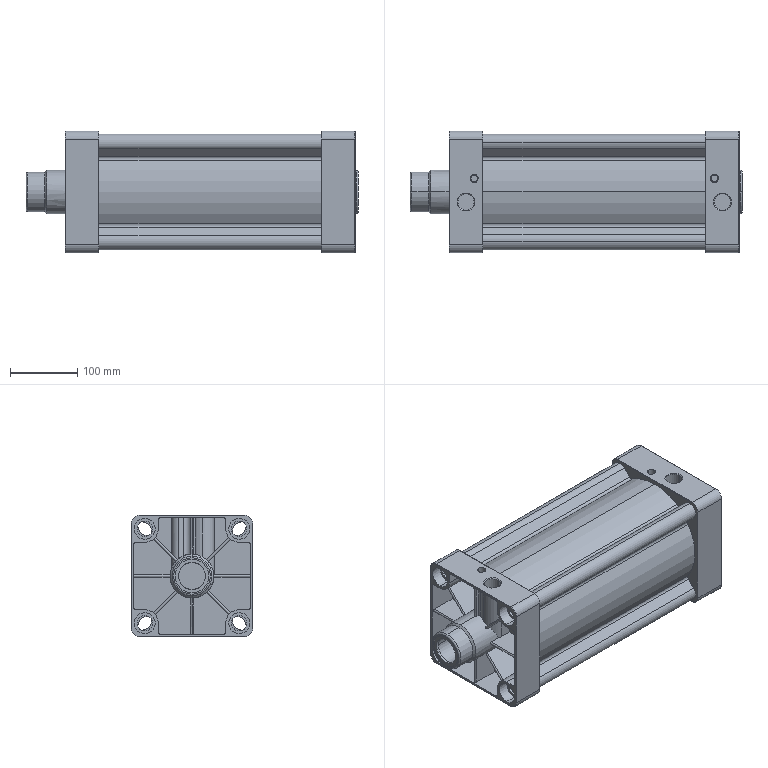Part | STEP file | 1 solid | 393 faces | box 492 x 180 x 180 mm | volume 3117873 mm3 | plane 186 | cylinder 173 | cone 30 | torus 4 | commonest cylinder face diameters 3.5 x18 6 x16 23 x16 31 x16 11 x12 10 x10